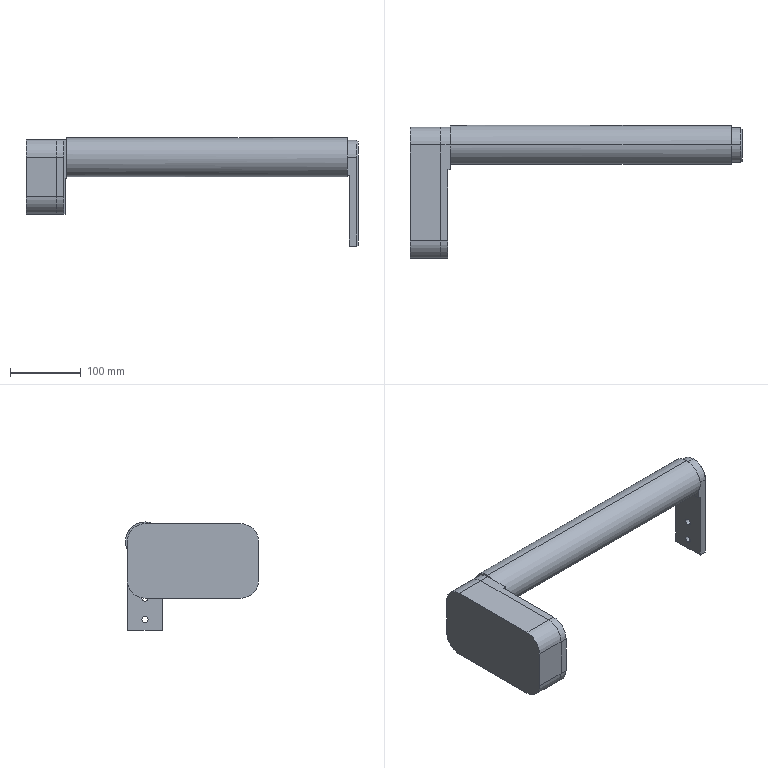Part | SolidWorks | features ICE 8, Chamfer 1, Extrusion 1, HoleWzd 1 | 2 solids | 59 faces | box 468 x 187.5 x 152.5 mm | volume 2041329 mm3 | plane 33 | cylinder 24 | cone 2 | commonest cylinder face diameters 50 x8 9 x4 15 x4 16 x2 30 x2 48 x2